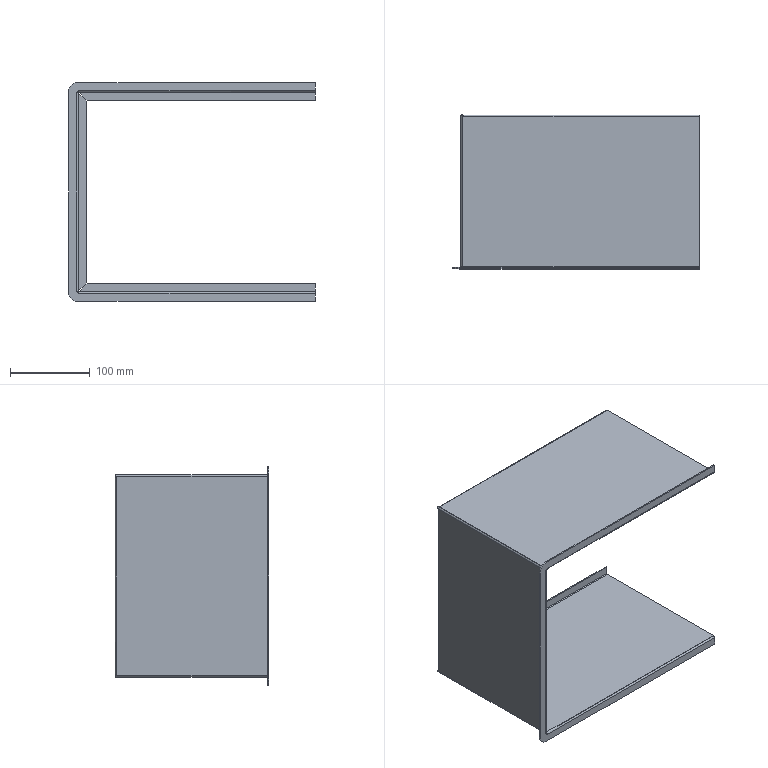Part | SolidWorks | features EdgeFlange 2, FlatPattern 1, ICE 1, MirrorPattern 1, SMBaseFlange 1, SheetMetal 1 | 1 solid | 74 faces | box 309 x 192.237 x 274 mm | volume 268790 mm3 | plane 50 | cylinder 20 | spline 4 | commonest cylinder face diameters 4.473 x10 1.473 x8 23.473 x2